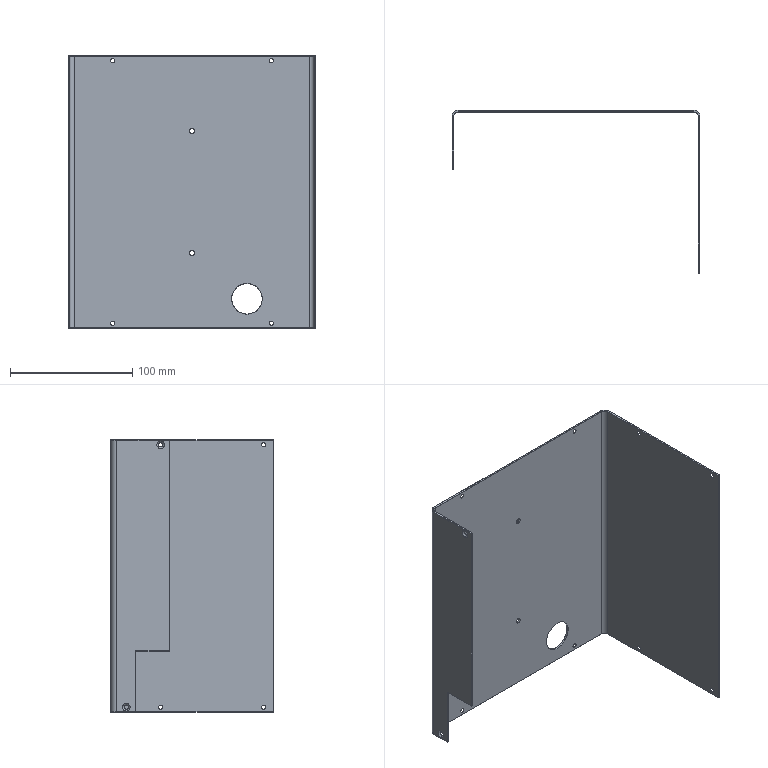Part | SolidWorks | features BaseBody 1 | 1 solid | 112 faces | box 203 x 133.5 x 222.9 mm | volume 123342 mm3 | plane 50 | cone 32 | cylinder 30 | commonest cylinder face diameters 3.4 x20 4.2 x4 7 x2 10 x2 25 x2